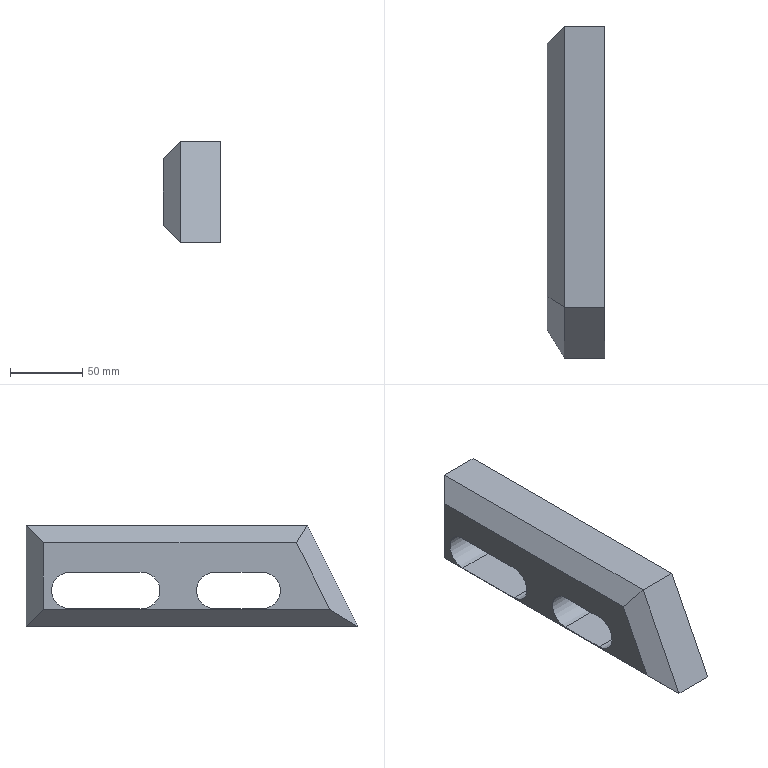Part | SolidWorks | features Chamfer 1, Extrusion 1 | 1 solid | 18 faces | box 40 x 229 x 70 mm | volume 431150 mm3 | plane 14 | cylinder 4 | commonest cylinder face diameters 25 x4
STEP:
#1=CARTESIAN_POINT('',(20.,114.,-32.5));
#2=VERTEX_POINT('',#1);
#3=CARTESIAN_POINT('',(20.,114.,-57.5));
#4=VERTEX_POINT('',#3);
#5=CARTESIAN_POINT('',(20.,114.,-45.));
#6=DIRECTION('',(1.,0.,0.));
#7=DIRECTION('',(0.,0.,-1.));
#8=AXIS2_PLACEMENT_3D('',#5,#6,#7);
#9=CIRCLE('',#8,12.5);
#10=EDGE_CURVE('',#2,#4,#9,.T.);
#11=ORIENTED_EDGE('',*,*,#10,.F.);
#12=CARTESIAN_POINT('',(20.,164.,-32.5));
#13=VERTEX_POINT('',#12);
#14=CARTESIAN_POINT('',(20.,114.,-32.5));
#15=DIRECTION('',(0.,-1.,0.));
#16=VECTOR('',#15,1000.);
#17=LINE('',#14,#16);
#18=EDGE_CURVE('',#13,#2,#17,.T.);
#19=ORIENTED_EDGE('',*,*,#18,.F.);
#20=CARTESIAN_POINT('',(20.,164.,-57.5));
#21=VERTEX_POINT('',#20);
#22=CARTESIAN_POINT('',(20.,164.,-45.));
#23=DIRECTION('',(1.,0.,0.));
#24=DIRECTION('',(0.,0.,-1.));
#25=AXIS2_PLACEMENT_3D('',#22,#23,#24);
#26=CIRCLE('',#25,12.5);
#27=EDGE_CURVE('',#21,#13,#26,.T.);
#28=ORIENTED_EDGE('',*,*,#27,.F.);
#29=CARTESIAN_POINT('',(20.,114.,-57.5));
#30=DIRECTION('',(0.,1.,0.));
#31=VECTOR('',#30,1000.);
#32=LINE('',#29,#31);
#33=EDGE_CURVE('',#4,#21,#32,.T.);
#34=ORIENTED_EDGE('',*,*,#33,.F.);
#35=EDGE_LOOP('',(#11,#19,#28,#34));
#36=FACE_BOUND('',#35,.T.);
#37=CARTESIAN_POINT('',(20.,194.,0.));
#38=VERTEX_POINT('',#37);
#39=CARTESIAN_POINT('',(20.,0.,0.));
#40=VERTEX_POINT('',#39);
#41=CARTESIAN_POINT('',(20.,194.,0.));
#42=DIRECTION('',(0.,-1.,0.));
#43=VECTOR('',#42,1000.);
#44=LINE('',#41,#43);
#45=EDGE_CURVE('',#38,#40,#44,.T.);
#46=ORIENTED_EDGE('',*,*,#45,.T.);
#47=CARTESIAN_POINT('',(20.,-35.,-70.));
#48=VERTEX_POINT('',#47);
#49=CARTESIAN_POINT('',(20.,0.,0.));
#50=DIRECTION('',(0.,-0.4472,-0.8944));
#51=VECTOR('',#50,1000.);
#52=LINE('',#49,#51);
#53=EDGE_CURVE('',#40,#48,#52,.T.);
#54=ORIENTED_EDGE('',*,*,#53,.T.);
#55=CARTESIAN_POINT('',(20.,194.,-70.));
#56=VERTEX_POINT('',#55);
#57=CARTESIAN_POINT('',(20.,-35.,-70.));
#58=DIRECTION('',(0.,1.,0.));
#59=VECTOR('',#58,1000.);
#60=LINE('',#57,#59);
#61=EDGE_CURVE('',#48,#56,#60,.T.);
#62=ORIENTED_EDGE('',*,*,#61,.T.);
#63=CARTESIAN_POINT('',(20.,194.,-70.));
#64=DIRECTION('',(0.,0.,1.));
#65=VECTOR('',#64,1000.);
#66=LINE('',#63,#65);
#67=EDGE_CURVE('',#56,#38,#66,.T.);
#68=ORIENTED_EDGE('',*,*,#67,.T.);
#69=EDGE_LOOP('',(#46,#54,#62,#68));
#70=FACE_OUTER_BOUND('',#69,.T.);
#71=CARTESIAN_POINT('',(20.,30.91,-32.5));
#72=VERTEX_POINT('',#71);
#73=CARTESIAN_POINT('',(20.,30.91,-57.5));
#74=VERTEX_POINT('',#73);
#75=CARTESIAN_POINT('',(20.,30.91,-45.));
#76=DIRECTION('',(1.,0.,0.));
#77=DIRECTION('',(0.,0.,-1.));
#78=AXIS2_PLACEMENT_3D('',#75,#76,#77);
#79=CIRCLE('',#78,12.5);
#80=EDGE_CURVE('',#72,#74,#79,.T.);
#81=ORIENTED_EDGE('',*,*,#80,.F.);
#82=CARTESIAN_POINT('',(20.,64.,-32.5));
#83=VERTEX_POINT('',#82);
#84=CARTESIAN_POINT('',(20.,30.91,-32.5));
#85=DIRECTION('',(0.,-1.,0.));
#86=VECTOR('',#85,1000.);
#87=LINE('',#84,#86);
#88=EDGE_CURVE('',#83,#72,#87,.T.);
#89=ORIENTED_EDGE('',*,*,#88,.F.);
#90=CARTESIAN_POINT('',(20.,64.,-57.5));
#91=VERTEX_POINT('',#90);
#92=CARTESIAN_POINT('',(20.,64.,-45.));
#93=DIRECTION('',(1.,0.,0.));
#94=DIRECTION('',(0.,0.,-1.));
#95=AXIS2_PLACEMENT_3D('',#92,#93,#94);
#96=CIRCLE('',#95,12.5);
#97=EDGE_CURVE('',#91,#83,#96,.T.);
#98=ORIENTED_EDGE('',*,*,#97,.F.);
#99=CARTESIAN_POINT('',(20.,30.91,-57.5));
#100=DIRECTION('',(0.,1.,0.));
#101=VECTOR('',#100,1000.);
#102=LINE('',#99,#101);
#103=EDGE_CURVE('',#74,#91,#102,.T.);
#104=ORIENTED_EDGE('',*,*,#103,.F.);
#105=EDGE_LOOP('',(#81,#89,#98,#104));
#106=FACE_BOUND('',#105,.T.);
#107=CARTESIAN_POINT('',(20.,0.,0.));
#108=DIRECTION('',(-1.,0.,0.));
#109=DIRECTION('',(0.,0.,1.));
#110=AXIS2_PLACEMENT_3D('',#107,#108,#109);
#111=PLANE('',#110);
#112=ADVANCED_FACE('',(#36,#70,#106),#111,.F.);
#113=CARTESIAN_POINT('',(-20.,182.,-12.));
#114=VERTEX_POINT('',#113);
#115=CARTESIAN_POINT('',(-20.,182.,-58.));
#116=VERTEX_POINT('',#115);
#117=CARTESIAN_POINT('',(-20.,182.,-70.));
#118=DIRECTION('',(0.,0.,-1.));
#119=VECTOR('',#118,1000.);
#120=LINE('',#117,#119);
#121=EDGE_CURVE('',#114,#116,#120,.T.);
#122=ORIENTED_EDGE('',*,*,#121,.T.);
#123=CARTESIAN_POINT('',(-20.,-15.584,-58.));
#124=VERTEX_POINT('',#123);
#125=CARTESIAN_POINT('',(-20.,-35.,-58.));
#126=DIRECTION('',(0.,-1.,0.));
#127=VECTOR('',#126,1000.);
#128=LINE('',#125,#127);
#129=EDGE_CURVE('',#116,#124,#128,.T.);
#130=ORIENTED_EDGE('',*,*,#129,.T.);
#131=CARTESIAN_POINT('',(-20.,7.416,-12.));
#132=VERTEX_POINT('',#131);
#133=CARTESIAN_POINT('',(-20.,10.733,-5.367));
#134=DIRECTION('',(0.,0.4472,0.8944));
#135=VECTOR('',#134,1000.);
#136=LINE('',#133,#135);
#137=EDGE_CURVE('',#124,#132,#136,.T.);
#138=ORIENTED_EDGE('',*,*,#137,.T.);
#139=CARTESIAN_POINT('',(-20.,194.,-12.));
#140=DIRECTION('',(0.,1.,0.));
#141=VECTOR('',#140,1000.);
#142=LINE('',#139,#141);
#143=EDGE_CURVE('',#132,#114,#142,.T.);
#144=ORIENTED_EDGE('',*,*,#143,.T.);
#145=EDGE_LOOP('',(#122,#130,#138,#144));
#146=FACE_OUTER_BOUND('',#145,.T.);
#147=CARTESIAN_POINT('',(-20.,164.,-32.5));
#148=VERTEX_POINT('',#147);
#149=CARTESIAN_POINT('',(-20.,114.,-32.5));
#150=VERTEX_POINT('',#149);
#151=CARTESIAN_POINT('',(-20.,114.,-32.5));
#152=DIRECTION('',(0.,-1.,0.));
#153=VECTOR('',#152,1000.);
#154=LINE('',#151,#153);
#155=EDGE_CURVE('',#148,#150,#154,.T.);
#156=ORIENTED_EDGE('',*,*,#155,.T.);
#157=CARTESIAN_POINT('',(-20.,114.,-57.5));
#158=VERTEX_POINT('',#157);
#159=CARTESIAN_POINT('',(-20.,114.,-45.));
#160=DIRECTION('',(1.,0.,0.));
#161=DIRECTION('',(0.,0.,-1.));
#162=AXIS2_PLACEMENT_3D('',#159,#160,#161);
#163=CIRCLE('',#162,12.5);
#164=EDGE_CURVE('',#150,#158,#163,.T.);
#165=ORIENTED_EDGE('',*,*,#164,.T.);
#166=CARTESIAN_POINT('',(-20.,164.,-57.5));
#167=VERTEX_POINT('',#166);
#168=CARTESIAN_POINT('',(-20.,114.,-57.5));
#169=DIRECTION('',(0.,1.,0.));
#170=VECTOR('',#169,1000.);
#171=LINE('',#168,#170);
#172=EDGE_CURVE('',#158,#167,#171,.T.);
#173=ORIENTED_EDGE('',*,*,#172,.T.);
#174=CARTESIAN_POINT('',(-20.,164.,-45.));
#175=DIRECTION('',(1.,0.,0.));
#176=DIRECTION('',(0.,0.,-1.));
#177=AXIS2_PLACEMENT_3D('',#174,#175,#176);
#178=CIRCLE('',#177,12.5);
#179=EDGE_CURVE('',#167,#148,#178,.T.);
#180=ORIENTED_EDGE('',*,*,#179,.T.);
#181=EDGE_LOOP('',(#156,#165,#173,#180));
#182=FACE_BOUND('',#181,.T.);
#183=CARTESIAN_POINT('',(-20.,64.,-32.5));
#184=VERTEX_POINT('',#183);
#185=CARTESIAN_POINT('',(-20.,30.91,-32.5));
#186=VERTEX_POINT('',#185);
#187=CARTESIAN_POINT('',(-20.,30.91,-32.5));
#188=DIRECTION('',(0.,-1.,0.));
#189=VECTOR('',#188,1000.);
#190=LINE('',#187,#189);
#191=EDGE_CURVE('',#184,#186,#190,.T.);
#192=ORIENTED_EDGE('',*,*,#191,.T.);
#193=CARTESIAN_POINT('',(-20.,30.91,-57.5));
#194=VERTEX_POINT('',#193);
#195=CARTESIAN_POINT('',(-20.,30.91,-45.));
#196=DIRECTION('',(1.,0.,0.));
#197=DIRECTION('',(0.,0.,-1.));
#198=AXIS2_PLACEMENT_3D('',#195,#196,#197);
#199=CIRCLE('',#198,12.5);
#200=EDGE_CURVE('',#186,#194,#199,.T.);
#201=ORIENTED_EDGE('',*,*,#200,.T.);
#202=CARTESIAN_POINT('',(-20.,64.,-57.5));
#203=VERTEX_POINT('',#202);
#204=CARTESIAN_POINT('',(-20.,30.91,-57.5));
#205=DIRECTION('',(0.,1.,0.));
#206=VECTOR('',#205,1000.);
#207=LINE('',#204,#206);
#208=EDGE_CURVE('',#194,#203,#207,.T.);
#209=ORIENTED_EDGE('',*,*,#208,.T.);
#210=CARTESIAN_POINT('',(-20.,64.,-45.));
#211=DIRECTION('',(1.,0.,0.));
#212=DIRECTION('',(0.,0.,-1.));
#213=AXIS2_PLACEMENT_3D('',#210,#211,#212);
#214=CIRCLE('',#213,12.5);
#215=EDGE_CURVE('',#203,#184,#214,.T.);
#216=ORIENTED_EDGE('',*,*,#215,.T.);
#217=EDGE_LOOP('',(#192,#201,#209,#216));
#218=FACE_BOUND('',#217,.T.);
#219=CARTESIAN_POINT('',(-20.,0.,0.));
#220=DIRECTION('',(-1.,0.,0.));
#221=DIRECTION('',(0.,0.,1.));
#222=AXIS2_PLACEMENT_3D('',#219,#220,#221);
#223=PLANE('',#222);
#224=ADVANCED_FACE('',(#146,#182,#218),#223,.T.);
#225=CARTESIAN_POINT('',(-8.,194.,0.));
#226=VERTEX_POINT('',#225);
#227=CARTESIAN_POINT('',(20.,194.,0.));
#228=DIRECTION('',(-1.,0.,0.));
#229=VECTOR('',#228,1000.);
#230=LINE('',#227,#229);
#231=EDGE_CURVE('',#38,#226,#230,.T.);
#232=ORIENTED_EDGE('',*,*,#231,.T.);
#233=CARTESIAN_POINT('',(-8.,0.,0.));
#234=VERTEX_POINT('',#233);
#235=CARTESIAN_POINT('',(-8.,0.,0.));
#236=DIRECTION('',(0.,-1.,0.));
#237=VECTOR('',#236,1000.);
#238=LINE('',#235,#237);
#239=EDGE_CURVE('',#226,#234,#238,.T.);
#240=ORIENTED_EDGE('',*,*,#239,.T.);
#241=CARTESIAN_POINT('',(20.,0.,0.));
#242=DIRECTION('',(-1.,0.,0.));
#243=VECTOR('',#242,1000.);
#244=LINE('',#241,#243);
#245=EDGE_CURVE('',#40,#234,#244,.T.);
#246=ORIENTED_EDGE('',*,*,#245,.F.);
#247=ORIENTED_EDGE('',*,*,#45,.F.);
#248=EDGE_LOOP('',(#232,#240,#246,#247));
#249=FACE_OUTER_BOUND('',#248,.T.);
#250=CARTESIAN_POINT('',(20.,194.,0.));
#251=DIRECTION('',(0.,0.,-1.));
#252=DIRECTION('',(-1.,0.,0.));
#253=AXIS2_PLACEMENT_3D('',#250,#251,#252);
#254=PLANE('',#253);
#255=ADVANCED_FACE('',(#249),#254,.F.);
#256=ORIENTED_EDGE('',*,*,#245,.T.);
#257=CARTESIAN_POINT('',(-8.,-35.,-70.));
#258=VERTEX_POINT('',#257);
#259=CARTESIAN_POINT('',(-8.,-35.,-70.));
#260=DIRECTION('',(0.,-0.4472,-0.8944));
#261=VECTOR('',#260,1000.);
#262=LINE('',#259,#261);
#263=EDGE_CURVE('',#234,#258,#262,.T.);
#264=ORIENTED_EDGE('',*,*,#263,.T.);
#265=CARTESIAN_POINT('',(20.,-35.,-70.));
#266=DIRECTION('',(-1.,0.,0.));
#267=VECTOR('',#266,1000.);
#268=LINE('',#265,#267);
#269=EDGE_CURVE('',#48,#258,#268,.T.);
#270=ORIENTED_EDGE('',*,*,#269,.F.);
#271=ORIENTED_EDGE('',*,*,#53,.F.);
#272=EDGE_LOOP('',(#256,#264,#270,#271));
#273=FACE_OUTER_BOUND('',#272,.T.);
#274=CARTESIAN_POINT('',(20.,0.,0.));
#275=DIRECTION('',(0.,0.8944,-0.4472));
#276=DIRECTION('',(0.,0.4472,0.8944));
#277=AXIS2_PLACEMENT_3D('',#274,#275,#276);
#278=PLANE('',#277);
#279=ADVANCED_FACE('',(#273),#278,.F.);
#280=ORIENTED_EDGE('',*,*,#269,.T.);
#281=CARTESIAN_POINT('',(-8.,194.,-70.));
#282=VERTEX_POINT('',#281);
#283=CARTESIAN_POINT('',(-8.,194.,-70.));
#284=DIRECTION('',(0.,1.,0.));
#285=VECTOR('',#284,1000.);
#286=LINE('',#283,#285);
#287=EDGE_CURVE('',#258,#282,#286,.T.);
#288=ORIENTED_EDGE('',*,*,#287,.T.);
#289=CARTESIAN_POINT('',(20.,194.,-70.));
#290=DIRECTION('',(-1.,0.,0.));
#291=VECTOR('',#290,1000.);
#292=LINE('',#289,#291);
#293=EDGE_CURVE('',#56,#282,#292,.T.);
#294=ORIENTED_EDGE('',*,*,#293,.F.);
#295=ORIENTED_EDGE('',*,*,#61,.F.);
#296=EDGE_LOOP('',(#280,#288,#294,#295));
#297=FACE_OUTER_BOUND('',#296,.T.);
#298=CARTESIAN_POINT('',(20.,-35.,-70.));
#299=DIRECTION('',(0.,0.,1.));
#300=DIRECTION('',(0.,-1.,0.));
#301=AXIS2_PLACEMENT_3D('',#298,#299,#300);
#302=PLANE('',#301);
#303=ADVANCED_FACE('',(#297),#302,.F.);
#304=ORIENTED_EDGE('',*,*,#293,.T.);
#305=CARTESIAN_POINT('',(-8.,194.,0.));
#306=DIRECTION('',(0.,0.,1.));
#307=VECTOR('',#306,1000.);
#308=LINE('',#305,#307);
#309=EDGE_CURVE('',#282,#226,#308,.T.);
#310=ORIENTED_EDGE('',*,*,#309,.T.);
#311=ORIENTED_EDGE('',*,*,#231,.F.);
#312=ORIENTED_EDGE('',*,*,#67,.F.);
#313=EDGE_LOOP('',(#304,#310,#311,#312));
#314=FACE_OUTER_BOUND('',#313,.T.);
#315=CARTESIAN_POINT('',(20.,194.,-70.));
#316=DIRECTION('',(0.,-1.,0.));
#317=DIRECTION('',(0.,0.,-1.));
#318=AXIS2_PLACEMENT_3D('',#315,#316,#317);
#319=PLANE('',#318);
#320=ADVANCED_FACE('',(#314),#319,.F.);
#321=ORIENTED_EDGE('',*,*,#164,.F.);
#322=CARTESIAN_POINT('',(20.,114.,-32.5));
#323=DIRECTION('',(-1.,0.,0.));
#324=VECTOR('',#323,1000.);
#325=LINE('',#322,#324);
#326=EDGE_CURVE('',#2,#150,#325,.T.);
#327=ORIENTED_EDGE('',*,*,#326,.F.);
#328=ORIENTED_EDGE('',*,*,#10,.T.);
#329=CARTESIAN_POINT('',(20.,114.,-57.5));
#330=DIRECTION('',(-1.,0.,0.));
#331=VECTOR('',#330,1000.);
#332=LINE('',#329,#331);
#333=EDGE_CURVE('',#4,#158,#332,.T.);
#334=ORIENTED_EDGE('',*,*,#333,.T.);
#335=EDGE_LOOP('',(#321,#327,#328,#334));
#336=FACE_OUTER_BOUND('',#335,.T.);
#337=CARTESIAN_POINT('',(20.,114.,-45.));
#338=DIRECTION('',(-1.,0.,0.));
#339=DIRECTION('',(0.,0.,1.));
#340=AXIS2_PLACEMENT_3D('',#337,#338,#339);
#341=CYLINDRICAL_SURFACE('',#340,12.5);
#342=ADVANCED_FACE('',(#336),#341,.F.);
#343=ORIENTED_EDGE('',*,*,#172,.F.);
#344=ORIENTED_EDGE('',*,*,#333,.F.);
#345=ORIENTED_EDGE('',*,*,#33,.T.);
#346=CARTESIAN_POINT('',(20.,164.,-57.5));
#347=DIRECTION('',(-1.,0.,0.));
#348=VECTOR('',#347,1000.);
#349=LINE('',#346,#348);
#350=EDGE_CURVE('',#21,#167,#349,.T.);
#351=ORIENTED_EDGE('',*,*,#350,.T.);
#352=EDGE_LOOP('',(#343,#344,#345,#351));
#353=FACE_OUTER_BOUND('',#352,.T.);
#354=CARTESIAN_POINT('',(20.,114.,-57.5));
#355=DIRECTION('',(0.,0.,1.));
#356=DIRECTION('',(1.,0.,0.));
#357=AXIS2_PLACEMENT_3D('',#354,#355,#356);
#358=PLANE('',#357);
#359=ADVANCED_FACE('',(#353),#358,.T.);
#360=ORIENTED_EDGE('',*,*,#179,.F.);
#361=ORIENTED_EDGE('',*,*,#350,.F.);
#362=ORIENTED_EDGE('',*,*,#27,.T.);
#363=CARTESIAN_POINT('',(20.,164.,-32.5));
#364=DIRECTION('',(-1.,0.,0.));
#365=VECTOR('',#364,1000.);
#366=LINE('',#363,#365);
#367=EDGE_CURVE('',#13,#148,#366,.T.);
#368=ORIENTED_EDGE('',*,*,#367,.T.);
#369=EDGE_LOOP('',(#360,#361,#362,#368));
#370=FACE_OUTER_BOUND('',#369,.T.);
#371=CARTESIAN_POINT('',(20.,164.,-45.));
#372=DIRECTION('',(-1.,0.,0.));
#373=DIRECTION('',(0.,0.,1.));
#374=AXIS2_PLACEMENT_3D('',#371,#372,#373);
#375=CYLINDRICAL_SURFACE('',#374,12.5);
#376=ADVANCED_FACE('',(#370),#375,.F.);
#377=ORIENTED_EDGE('',*,*,#155,.F.);
#378=ORIENTED_EDGE('',*,*,#367,.F.);
#379=ORIENTED_EDGE('',*,*,#18,.T.);
#380=ORIENTED_EDGE('',*,*,#326,.T.);
#381=EDGE_LOOP('',(#377,#378,#379,#380));
#382=FACE_OUTER_BOUND('',#381,.T.);
#383=CARTESIAN_POINT('',(20.,114.,-32.5));
#384=DIRECTION('',(0.,0.,-1.));
#385=DIRECTION('',(-1.,0.,0.));
#386=AXIS2_PLACEMENT_3D('',#383,#384,#385);
#387=PLANE('',#386);
#388=ADVANCED_FACE('',(#382),#387,.T.);
#389=ORIENTED_EDGE('',*,*,#200,.F.);
#390=CARTESIAN_POINT('',(20.,30.91,-32.5));
#391=DIRECTION('',(-1.,0.,0.));
#392=VECTOR('',#391,1000.);
#393=LINE('',#390,#392);
#394=EDGE_CURVE('',#72,#186,#393,.T.);
#395=ORIENTED_EDGE('',*,*,#394,.F.);
#396=ORIENTED_EDGE('',*,*,#80,.T.);
#397=CARTESIAN_POINT('',(20.,30.91,-57.5));
#398=DIRECTION('',(-1.,0.,0.));
#399=VECTOR('',#398,1000.);
#400=LINE('',#397,#399);
#401=EDGE_CURVE('',#74,#194,#400,.T.);
#402=ORIENTED_EDGE('',*,*,#401,.T.);
#403=EDGE_LOOP('',(#389,#395,#396,#402));
#404=FACE_OUTER_BOUND('',#403,.T.);
#405=CARTESIAN_POINT('',(20.,30.91,-45.));
#406=DIRECTION('',(-1.,0.,0.));
#407=DIRECTION('',(0.,0.,1.));
#408=AXIS2_PLACEMENT_3D('',#405,#406,#407);
#409=CYLINDRICAL_SURFACE('',#408,12.5);
#410=ADVANCED_FACE('',(#404),#409,.F.);
#411=ORIENTED_EDGE('',*,*,#208,.F.);
#412=ORIENTED_EDGE('',*,*,#401,.F.);
#413=ORIENTED_EDGE('',*,*,#103,.T.);
#414=CARTESIAN_POINT('',(20.,64.,-57.5));
#415=DIRECTION('',(-1.,0.,0.));
#416=VECTOR('',#415,1000.);
#417=LINE('',#414,#416);
#418=EDGE_CURVE('',#91,#203,#417,.T.);
#419=ORIENTED_EDGE('',*,*,#418,.T.);
#420=EDGE_LOOP('',(#411,#412,#413,#419));
#421=FACE_OUTER_BOUND('',#420,.T.);
#422=CARTESIAN_POINT('',(20.,30.91,-57.5));
#423=DIRECTION('',(0.,0.,1.));
#424=DIRECTION('',(1.,0.,0.));
#425=AXIS2_PLACEMENT_3D('',#422,#423,#424);
#426=PLANE('',#425);
#427=ADVANCED_FACE('',(#421),#426,.T.);
#428=ORIENTED_EDGE('',*,*,#215,.F.);
#429=ORIENTED_EDGE('',*,*,#418,.F.);
#430=ORIENTED_EDGE('',*,*,#97,.T.);
#431=CARTESIAN_POINT('',(20.,64.,-32.5));
#432=DIRECTION('',(-1.,0.,0.));
#433=VECTOR('',#432,1000.);
#434=LINE('',#431,#433);
#435=EDGE_CURVE('',#83,#184,#434,.T.);
#436=ORIENTED_EDGE('',*,*,#435,.T.);
#437=EDGE_LOOP('',(#428,#429,#430,#436));
#438=FACE_OUTER_BOUND('',#437,.T.);
#439=CARTESIAN_POINT('',(20.,64.,-45.));
#440=DIRECTION('',(-1.,0.,0.));
#441=DIRECTION('',(0.,0.,1.));
#442=AXIS2_PLACEMENT_3D('',#439,#440,#441);
#443=CYLINDRICAL_SURFACE('',#442,12.5);
#444=ADVANCED_FACE('',(#438),#443,.F.);
#445=ORIENTED_EDGE('',*,*,#191,.F.);
#446=ORIENTED_EDGE('',*,*,#435,.F.);
#447=ORIENTED_EDGE('',*,*,#88,.T.);
#448=ORIENTED_EDGE('',*,*,#394,.T.);
#449=EDGE_LOOP('',(#445,#446,#447,#448));
#450=FACE_OUTER_BOUND('',#449,.T.);
#451=CARTESIAN_POINT('',(20.,30.91,-32.5));
#452=DIRECTION('',(0.,0.,-1.));
#453=DIRECTION('',(-1.,0.,0.));
#454=AXIS2_PLACEMENT_3D('',#451,#452,#453);
#455=PLANE('',#454);
#456=ADVANCED_FACE('',(#450),#455,.T.);
#457=CARTESIAN_POINT('',(-8.,194.,0.));
#458=DIRECTION('',(0.5774,0.5774,0.5774));
#459=VECTOR('',#458,1000.);
#460=LINE('',#457,#459);
#461=EDGE_CURVE('',#114,#226,#460,.T.);
#462=ORIENTED_EDGE('',*,*,#461,.F.);
#463=ORIENTED_EDGE('',*,*,#143,.F.);
#464=CARTESIAN_POINT('',(-8.,0.,0.));
#465=DIRECTION('',(-0.6479,0.4004,-0.6479));
#466=VECTOR('',#465,1000.);
#467=LINE('',#464,#466);
#468=EDGE_CURVE('',#234,#132,#467,.T.);
#469=ORIENTED_EDGE('',*,*,#468,.F.);
#470=ORIENTED_EDGE('',*,*,#239,.F.);
#471=EDGE_LOOP('',(#462,#463,#469,#470));
#472=FACE_OUTER_BOUND('',#471,.T.);
#473=CARTESIAN_POINT('',(-8.,194.,0.));
#474=DIRECTION('',(-0.7071,0.,0.7071));
#475=DIRECTION('',(0.,1.,0.));
#476=AXIS2_PLACEMENT_3D('',#473,#474,#475);
#477=PLANE('',#476);
#478=ADVANCED_FACE('',(#472),#477,.T.);
#479=ORIENTED_EDGE('',*,*,#468,.T.);
#480=ORIENTED_EDGE('',*,*,#137,.F.);
#481=CARTESIAN_POINT('',(-35.421,9.368,-42.579));
#482=DIRECTION('',(-0.4653,0.7529,0.4653));
#483=VECTOR('',#482,1000.);
#484=LINE('',#481,#483);
#485=EDGE_CURVE('',#258,#124,#484,.T.);
#486=ORIENTED_EDGE('',*,*,#485,.F.);
#487=ORIENTED_EDGE('',*,*,#263,.F.);
#488=EDGE_LOOP('',(#479,#480,#486,#487));
#489=FACE_OUTER_BOUND('',#488,.T.);
#490=CARTESIAN_POINT('',(-8.,0.,0.));
#491=DIRECTION('',(-0.7071,-0.6325,0.3162));
#492=DIRECTION('',(0.,0.4472,0.8944));
#493=AXIS2_PLACEMENT_3D('',#490,#491,#492);
#494=PLANE('',#493);
#495=ADVANCED_FACE('',(#489),#494,.T.);
#496=ORIENTED_EDGE('',*,*,#461,.T.);
#497=ORIENTED_EDGE('',*,*,#309,.F.);
#498=CARTESIAN_POINT('',(-8.,194.,-70.));
#499=DIRECTION('',(0.5774,0.5774,-0.5774));
#500=VECTOR('',#499,1000.);
#501=LINE('',#498,#500);
#502=EDGE_CURVE('',#116,#282,#501,.T.);
#503=ORIENTED_EDGE('',*,*,#502,.F.);
#504=ORIENTED_EDGE('',*,*,#121,.F.);
#505=EDGE_LOOP('',(#496,#497,#503,#504));
#506=FACE_OUTER_BOUND('',#505,.T.);
#507=CARTESIAN_POINT('',(-8.,194.,-70.));
#508=DIRECTION('',(-0.7071,0.7071,0.));
#509=DIRECTION('',(0.,0.,-1.));
#510=AXIS2_PLACEMENT_3D('',#507,#508,#509);
#511=PLANE('',#510);
#512=ADVANCED_FACE('',(#506),#511,.T.);
#513=ORIENTED_EDGE('',*,*,#485,.T.);
#514=ORIENTED_EDGE('',*,*,#129,.F.);
#515=ORIENTED_EDGE('',*,*,#502,.T.);
#516=ORIENTED_EDGE('',*,*,#287,.F.);
#517=EDGE_LOOP('',(#513,#514,#515,#516));
#518=FACE_OUTER_BOUND('',#517,.T.);
#519=CARTESIAN_POINT('',(-8.,-35.,-70.));
#520=DIRECTION('',(-0.7071,0.,-0.7071));
#521=DIRECTION('',(0.,-1.,0.));
#522=AXIS2_PLACEMENT_3D('',#519,#520,#521);
#523=PLANE('',#522);
#524=ADVANCED_FACE('',(#518),#523,.T.);
#525=CLOSED_SHELL('',(#112,#224,#255,#279,#303,#320,#342,#359,#376,#388,#410,#427,#444,#456,#478,#495,#512,#524));
#526=MANIFOLD_SOLID_BREP('',#525);
#527=CARTESIAN_POINT('',(0.,0.,0.));
#528=DIRECTION('',(0.,0.,1.));
#529=DIRECTION('',(1.,0.,0.));
#530=AXIS2_PLACEMENT_3D('',#527,#528,#529);
#531=(LENGTH_UNIT()NAMED_UNIT(*)SI_UNIT(.MILLI.,.METRE.));
#532=UNCERTAINTY_MEASURE_WITH_UNIT(LENGTH_MEASURE(0.00001),#531,'','');
#533=(NAMED_UNIT(*)PLANE_ANGLE_UNIT()SI_UNIT($,.RADIAN.));
#534=(NAMED_UNIT(*)SI_UNIT($,.STERADIAN.)SOLID_ANGLE_UNIT());
#535=(GEOMETRIC_REPRESENTATION_CONTEXT(3)GLOBAL_UNCERTAINTY_ASSIGNED_CONTEXT((#532))GLOBAL_UNIT_ASSIGNED_CONTEXT((#531,#533,#534))REPRESENTATION_CONTEXT('',''));
#536=ADVANCED_BREP_SHAPE_REPRESENTATION('',(#526,#530),#535);